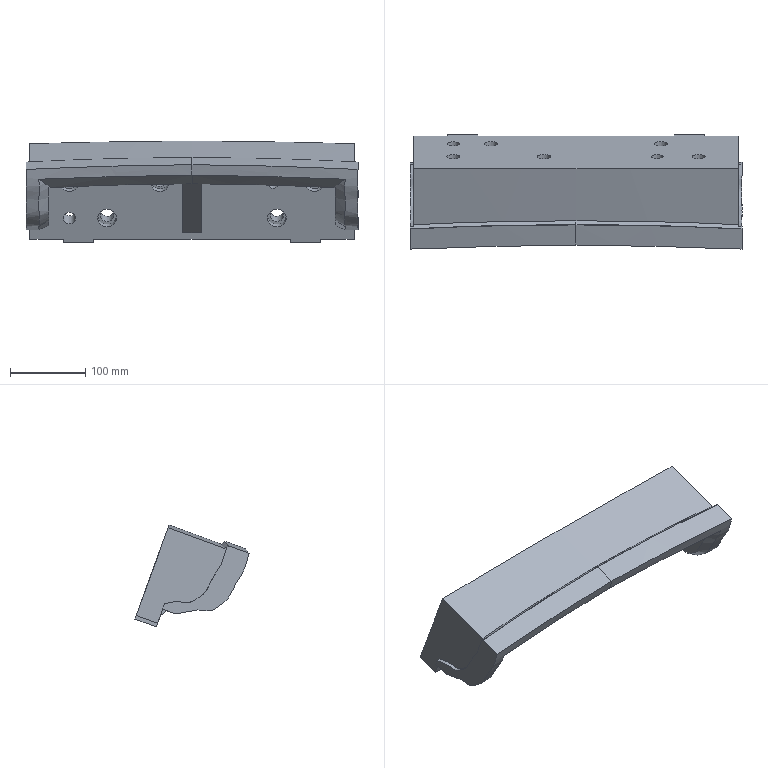Part | NX | features solid 2 | 1 solid | 57 faces | box 440 x 151.34 x 134.801 mm | volume 2811479 mm3 | plane 29 | spline 16 | cylinder 12 | commonest cylinder face diameters 17.5 x5 25 x5 16 x2